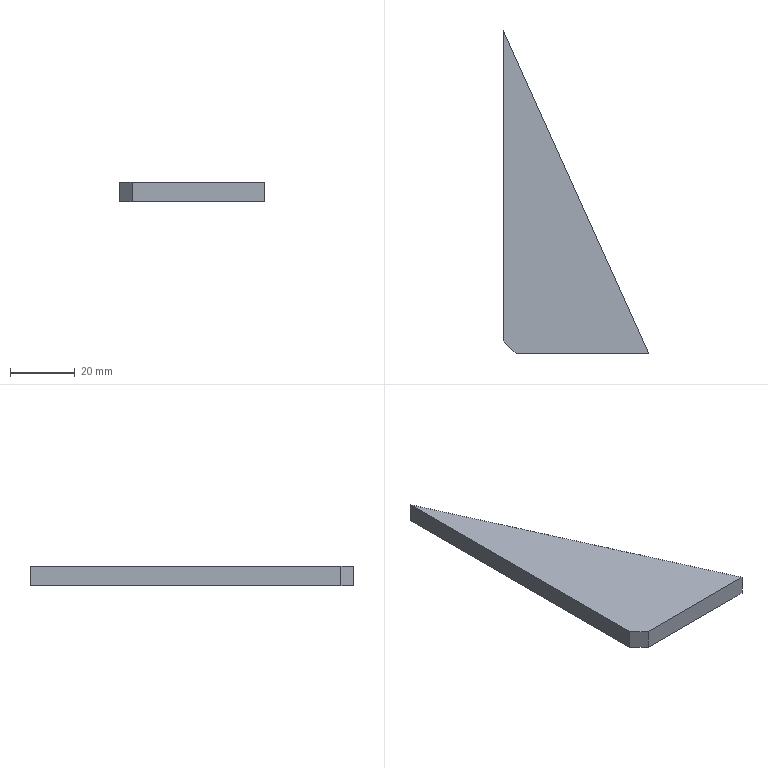Part | STEP file | BCC3 H14_6B | 1 solid | 6 faces | box 45 x 100 x 6 mm | volume 13452 mm3 | plane 6
STEP:
#1=CARTESIAN_POINT('',(0.,0.,0.));
#2=DIRECTION('',(0.,0.,1.));
#3=DIRECTION('',(1.,0.,0.));
#4=AXIS2_PLACEMENT_3D('',#1,#2,#3);
#5=CARTESIAN_POINT('',(4.,0.,6.));
#6=VERTEX_POINT('',#5);
#7=CARTESIAN_POINT('',(45.,0.,6.));
#8=VERTEX_POINT('',#7);
#9=CARTESIAN_POINT('',(45.,0.,6.));
#10=DIRECTION('',(1.,0.,0.));
#11=VECTOR('',#10,1.);
#12=LINE('',#9,#11);
#13=CARTESIAN_POINT('',(45.,0.,6.));
#14=DIRECTION('',(0.,1.,0.));
#15=DIRECTION('',(-1.,0.,0.));
#16=AXIS2_PLACEMENT_3D('',#13,#14,#15);
#17=PLANE('',#16);
#18=CARTESIAN_POINT('',(0.,0.));
#19=DIRECTION('',(-1.,0.));
#20=VECTOR('',#19,1.);
#21=LINE('',#18,#20);
#22=(GEOMETRIC_REPRESENTATION_CONTEXT(2)PARAMETRIC_REPRESENTATION_CONTEXT()REPRESENTATION_CONTEXT('',''));
#23=DEFINITIONAL_REPRESENTATION('',(#21),#22);
#24=PCURVE('',#17,#23);
#25=CARTESIAN_POINT('',(0.,0.,6.));
#26=DIRECTION('',(0.,0.,-1.));
#27=DIRECTION('',(-1.,0.,0.));
#28=AXIS2_PLACEMENT_3D('',#25,#26,#27);
#29=PLANE('',#28);
#30=CARTESIAN_POINT('',(-45.,0.));
#31=DIRECTION('',(-1.,0.));
#32=VECTOR('',#31,1.);
#33=LINE('',#30,#32);
#34=(GEOMETRIC_REPRESENTATION_CONTEXT(2)PARAMETRIC_REPRESENTATION_CONTEXT()REPRESENTATION_CONTEXT('',''));
#35=DEFINITIONAL_REPRESENTATION('',(#33),#34);
#36=PCURVE('',#29,#35);
#37=SURFACE_CURVE('',#12,(#24,#36),.PCURVE_S1.);
#38=EDGE_CURVE('',#6,#8,#37,.T.);
#39=ORIENTED_EDGE('',*,*,#38,.F.);
#40=CARTESIAN_POINT('',(4.,0.,0.));
#41=VERTEX_POINT('',#40);
#42=CARTESIAN_POINT('',(4.,0.,6.));
#43=DIRECTION('',(0.,0.,-1.));
#44=VECTOR('',#43,1.);
#45=LINE('',#42,#44);
#46=CARTESIAN_POINT('',(41.,0.));
#47=DIRECTION('',(0.,-1.));
#48=VECTOR('',#47,1.);
#49=LINE('',#46,#48);
#50=(GEOMETRIC_REPRESENTATION_CONTEXT(2)PARAMETRIC_REPRESENTATION_CONTEXT()REPRESENTATION_CONTEXT('',''));
#51=DEFINITIONAL_REPRESENTATION('',(#49),#50);
#52=PCURVE('',#17,#51);
#53=CARTESIAN_POINT('',(4.,0.,6.));
#54=DIRECTION('',(0.7071,0.7071,0.));
#55=DIRECTION('',(0.,0.,-1.));
#56=AXIS2_PLACEMENT_3D('',#53,#54,#55);
#57=PLANE('',#56);
#58=CARTESIAN_POINT('',(0.,0.));
#59=DIRECTION('',(1.,0.));
#60=VECTOR('',#59,1.);
#61=LINE('',#58,#60);
#62=(GEOMETRIC_REPRESENTATION_CONTEXT(2)PARAMETRIC_REPRESENTATION_CONTEXT()REPRESENTATION_CONTEXT('',''));
#63=DEFINITIONAL_REPRESENTATION('',(#61),#62);
#64=PCURVE('',#57,#63);
#65=SURFACE_CURVE('',#45,(#52,#64),.PCURVE_S1.);
#66=EDGE_CURVE('',#6,#41,#65,.T.);
#67=ORIENTED_EDGE('',*,*,#66,.T.);
#68=CARTESIAN_POINT('',(45.,0.,0.));
#69=VERTEX_POINT('',#68);
#70=CARTESIAN_POINT('',(45.,0.,0.));
#71=DIRECTION('',(1.,0.,0.));
#72=VECTOR('',#71,1.);
#73=LINE('',#70,#72);
#74=CARTESIAN_POINT('',(0.,-6.));
#75=DIRECTION('',(-1.,0.));
#76=VECTOR('',#75,1.);
#77=LINE('',#74,#76);
#78=(GEOMETRIC_REPRESENTATION_CONTEXT(2)PARAMETRIC_REPRESENTATION_CONTEXT()REPRESENTATION_CONTEXT('',''));
#79=DEFINITIONAL_REPRESENTATION('',(#77),#78);
#80=PCURVE('',#17,#79);
#81=CARTESIAN_POINT('',(0.,0.,0.));
#82=DIRECTION('',(0.,0.,-1.));
#83=DIRECTION('',(-1.,0.,0.));
#84=AXIS2_PLACEMENT_3D('',#81,#82,#83);
#85=PLANE('',#84);
#86=CARTESIAN_POINT('',(-45.,0.));
#87=DIRECTION('',(-1.,0.));
#88=VECTOR('',#87,1.);
#89=LINE('',#86,#88);
#90=(GEOMETRIC_REPRESENTATION_CONTEXT(2)PARAMETRIC_REPRESENTATION_CONTEXT()REPRESENTATION_CONTEXT('',''));
#91=DEFINITIONAL_REPRESENTATION('',(#89),#90);
#92=PCURVE('',#85,#91);
#93=SURFACE_CURVE('',#73,(#80,#92),.PCURVE_S1.);
#94=EDGE_CURVE('',#41,#69,#93,.T.);
#95=ORIENTED_EDGE('',*,*,#94,.T.);
#96=CARTESIAN_POINT('',(45.,0.,6.));
#97=DIRECTION('',(0.,0.,-1.));
#98=VECTOR('',#97,1.);
#99=LINE('',#96,#98);
#100=CARTESIAN_POINT('',(0.,0.));
#101=DIRECTION('',(0.,-1.));
#102=VECTOR('',#101,1.);
#103=LINE('',#100,#102);
#104=(GEOMETRIC_REPRESENTATION_CONTEXT(2)PARAMETRIC_REPRESENTATION_CONTEXT()REPRESENTATION_CONTEXT('',''));
#105=DEFINITIONAL_REPRESENTATION('',(#103),#104);
#106=PCURVE('',#17,#105);
#107=CARTESIAN_POINT('',(0.,100.,6.));
#108=DIRECTION('',(-0.9119,-0.4104,0.));
#109=DIRECTION('',(0.4104,-0.9119,0.));
#110=AXIS2_PLACEMENT_3D('',#107,#108,#109);
#111=PLANE('',#110);
#112=CARTESIAN_POINT('',(109.659,0.));
#113=DIRECTION('',(0.,-1.));
#114=VECTOR('',#113,1.);
#115=LINE('',#112,#114);
#116=(GEOMETRIC_REPRESENTATION_CONTEXT(2)PARAMETRIC_REPRESENTATION_CONTEXT()REPRESENTATION_CONTEXT('',''));
#117=DEFINITIONAL_REPRESENTATION('',(#115),#116);
#118=PCURVE('',#111,#117);
#119=SURFACE_CURVE('',#99,(#106,#118),.PCURVE_S1.);
#120=EDGE_CURVE('',#8,#69,#119,.T.);
#121=ORIENTED_EDGE('',*,*,#120,.F.);
#122=EDGE_LOOP('',(#39,#67,#95,#121));
#123=FACE_BOUND('',#122,.T.);
#124=ADVANCED_FACE('',(#123),#17,.F.);
#125=CARTESIAN_POINT('',(0.,100.,0.));
#126=VERTEX_POINT('',#125);
#127=CARTESIAN_POINT('',(0.,100.,0.));
#128=DIRECTION('',(-0.4104,0.9119,0.));
#129=VECTOR('',#128,1.);
#130=LINE('',#127,#129);
#131=CARTESIAN_POINT('',(0.,-6.));
#132=DIRECTION('',(-1.,0.));
#133=VECTOR('',#132,1.);
#134=LINE('',#131,#133);
#135=(GEOMETRIC_REPRESENTATION_CONTEXT(2)PARAMETRIC_REPRESENTATION_CONTEXT()REPRESENTATION_CONTEXT('',''));
#136=DEFINITIONAL_REPRESENTATION('',(#134),#135);
#137=PCURVE('',#111,#136);
#138=CARTESIAN_POINT('',(0.,100.));
#139=DIRECTION('',(0.4104,0.9119));
#140=VECTOR('',#139,1.);
#141=LINE('',#138,#140);
#142=(GEOMETRIC_REPRESENTATION_CONTEXT(2)PARAMETRIC_REPRESENTATION_CONTEXT()REPRESENTATION_CONTEXT('',''));
#143=DEFINITIONAL_REPRESENTATION('',(#141),#142);
#144=PCURVE('',#85,#143);
#145=SURFACE_CURVE('',#130,(#137,#144),.PCURVE_S1.);
#146=EDGE_CURVE('',#69,#126,#145,.T.);
#147=ORIENTED_EDGE('',*,*,#146,.T.);
#148=CARTESIAN_POINT('',(0.,100.,6.));
#149=VERTEX_POINT('',#148);
#150=CARTESIAN_POINT('',(0.,100.,6.));
#151=DIRECTION('',(0.,0.,-1.));
#152=VECTOR('',#151,1.);
#153=LINE('',#150,#152);
#154=CARTESIAN_POINT('',(0.,0.));
#155=DIRECTION('',(0.,-1.));
#156=VECTOR('',#155,1.);
#157=LINE('',#154,#156);
#158=(GEOMETRIC_REPRESENTATION_CONTEXT(2)PARAMETRIC_REPRESENTATION_CONTEXT()REPRESENTATION_CONTEXT('',''));
#159=DEFINITIONAL_REPRESENTATION('',(#157),#158);
#160=PCURVE('',#111,#159);
#161=CARTESIAN_POINT('',(0.,0.,6.));
#162=DIRECTION('',(1.,0.,0.));
#163=DIRECTION('',(0.,0.,-1.));
#164=AXIS2_PLACEMENT_3D('',#161,#162,#163);
#165=PLANE('',#164);
#166=CARTESIAN_POINT('',(0.,100.));
#167=DIRECTION('',(1.,0.));
#168=VECTOR('',#167,1.);
#169=LINE('',#166,#168);
#170=(GEOMETRIC_REPRESENTATION_CONTEXT(2)PARAMETRIC_REPRESENTATION_CONTEXT()REPRESENTATION_CONTEXT('',''));
#171=DEFINITIONAL_REPRESENTATION('',(#169),#170);
#172=PCURVE('',#165,#171);
#173=SURFACE_CURVE('',#153,(#160,#172),.PCURVE_S1.);
#174=EDGE_CURVE('',#149,#126,#173,.T.);
#175=ORIENTED_EDGE('',*,*,#174,.F.);
#176=CARTESIAN_POINT('',(0.,100.,6.));
#177=DIRECTION('',(-0.4104,0.9119,0.));
#178=VECTOR('',#177,1.);
#179=LINE('',#176,#178);
#180=CARTESIAN_POINT('',(0.,0.));
#181=DIRECTION('',(-1.,0.));
#182=VECTOR('',#181,1.);
#183=LINE('',#180,#182);
#184=(GEOMETRIC_REPRESENTATION_CONTEXT(2)PARAMETRIC_REPRESENTATION_CONTEXT()REPRESENTATION_CONTEXT('',''));
#185=DEFINITIONAL_REPRESENTATION('',(#183),#184);
#186=PCURVE('',#111,#185);
#187=CARTESIAN_POINT('',(0.,100.));
#188=DIRECTION('',(0.4104,0.9119));
#189=VECTOR('',#188,1.);
#190=LINE('',#187,#189);
#191=(GEOMETRIC_REPRESENTATION_CONTEXT(2)PARAMETRIC_REPRESENTATION_CONTEXT()REPRESENTATION_CONTEXT('',''));
#192=DEFINITIONAL_REPRESENTATION('',(#190),#191);
#193=PCURVE('',#29,#192);
#194=SURFACE_CURVE('',#179,(#186,#193),.PCURVE_S1.);
#195=EDGE_CURVE('',#8,#149,#194,.T.);
#196=ORIENTED_EDGE('',*,*,#195,.F.);
#197=ORIENTED_EDGE('',*,*,#120,.T.);
#198=EDGE_LOOP('',(#147,#175,#196,#197));
#199=FACE_BOUND('',#198,.T.);
#200=ADVANCED_FACE('',(#199),#111,.F.);
#201=CARTESIAN_POINT('',(0.,4.,0.));
#202=VERTEX_POINT('',#201);
#203=CARTESIAN_POINT('',(0.,0.,0.));
#204=DIRECTION('',(0.,-1.,0.));
#205=VECTOR('',#204,1.);
#206=LINE('',#203,#205);
#207=CARTESIAN_POINT('',(6.,0.));
#208=DIRECTION('',(0.,-1.));
#209=VECTOR('',#208,1.);
#210=LINE('',#207,#209);
#211=(GEOMETRIC_REPRESENTATION_CONTEXT(2)PARAMETRIC_REPRESENTATION_CONTEXT()REPRESENTATION_CONTEXT('',''));
#212=DEFINITIONAL_REPRESENTATION('',(#210),#211);
#213=PCURVE('',#165,#212);
#214=CARTESIAN_POINT('',(0.,0.));
#215=DIRECTION('',(0.,-1.));
#216=VECTOR('',#215,1.);
#217=LINE('',#214,#216);
#218=(GEOMETRIC_REPRESENTATION_CONTEXT(2)PARAMETRIC_REPRESENTATION_CONTEXT()REPRESENTATION_CONTEXT('',''));
#219=DEFINITIONAL_REPRESENTATION('',(#217),#218);
#220=PCURVE('',#85,#219);
#221=SURFACE_CURVE('',#206,(#213,#220),.PCURVE_S1.);
#222=EDGE_CURVE('',#126,#202,#221,.T.);
#223=ORIENTED_EDGE('',*,*,#222,.T.);
#224=CARTESIAN_POINT('',(0.,4.,6.));
#225=VERTEX_POINT('',#224);
#226=CARTESIAN_POINT('',(0.,4.,6.));
#227=DIRECTION('',(0.,0.,1.));
#228=VECTOR('',#227,1.);
#229=LINE('',#226,#228);
#230=CARTESIAN_POINT('',(0.,4.));
#231=DIRECTION('',(-1.,0.));
#232=VECTOR('',#231,1.);
#233=LINE('',#230,#232);
#234=(GEOMETRIC_REPRESENTATION_CONTEXT(2)PARAMETRIC_REPRESENTATION_CONTEXT()REPRESENTATION_CONTEXT('',''));
#235=DEFINITIONAL_REPRESENTATION('',(#233),#234);
#236=PCURVE('',#165,#235);
#237=CARTESIAN_POINT('',(0.,5.657));
#238=DIRECTION('',(-1.,0.));
#239=VECTOR('',#238,1.);
#240=LINE('',#237,#239);
#241=(GEOMETRIC_REPRESENTATION_CONTEXT(2)PARAMETRIC_REPRESENTATION_CONTEXT()REPRESENTATION_CONTEXT('',''));
#242=DEFINITIONAL_REPRESENTATION('',(#240),#241);
#243=PCURVE('',#57,#242);
#244=SURFACE_CURVE('',#229,(#236,#243),.PCURVE_S1.);
#245=EDGE_CURVE('',#202,#225,#244,.T.);
#246=ORIENTED_EDGE('',*,*,#245,.T.);
#247=CARTESIAN_POINT('',(0.,0.,6.));
#248=DIRECTION('',(0.,-1.,0.));
#249=VECTOR('',#248,1.);
#250=LINE('',#247,#249);
#251=CARTESIAN_POINT('',(0.,0.));
#252=DIRECTION('',(0.,-1.));
#253=VECTOR('',#252,1.);
#254=LINE('',#251,#253);
#255=(GEOMETRIC_REPRESENTATION_CONTEXT(2)PARAMETRIC_REPRESENTATION_CONTEXT()REPRESENTATION_CONTEXT('',''));
#256=DEFINITIONAL_REPRESENTATION('',(#254),#255);
#257=PCURVE('',#165,#256);
#258=CARTESIAN_POINT('',(0.,0.));
#259=DIRECTION('',(0.,-1.));
#260=VECTOR('',#259,1.);
#261=LINE('',#258,#260);
#262=(GEOMETRIC_REPRESENTATION_CONTEXT(2)PARAMETRIC_REPRESENTATION_CONTEXT()REPRESENTATION_CONTEXT('',''));
#263=DEFINITIONAL_REPRESENTATION('',(#261),#262);
#264=PCURVE('',#29,#263);
#265=SURFACE_CURVE('',#250,(#257,#264),.PCURVE_S1.);
#266=EDGE_CURVE('',#149,#225,#265,.T.);
#267=ORIENTED_EDGE('',*,*,#266,.F.);
#268=ORIENTED_EDGE('',*,*,#174,.T.);
#269=EDGE_LOOP('',(#223,#246,#267,#268));
#270=FACE_BOUND('',#269,.T.);
#271=ADVANCED_FACE('',(#270),#165,.F.);
#272=ORIENTED_EDGE('',*,*,#266,.T.);
#273=CARTESIAN_POINT('',(4.,0.,6.));
#274=DIRECTION('',(0.7071,-0.7071,0.));
#275=VECTOR('',#274,1.);
#276=LINE('',#273,#275);
#277=CARTESIAN_POINT('',(-4.,0.));
#278=DIRECTION('',(-0.7071,-0.7071));
#279=VECTOR('',#278,1.);
#280=LINE('',#277,#279);
#281=(GEOMETRIC_REPRESENTATION_CONTEXT(2)PARAMETRIC_REPRESENTATION_CONTEXT()REPRESENTATION_CONTEXT('',''));
#282=DEFINITIONAL_REPRESENTATION('',(#280),#281);
#283=PCURVE('',#29,#282);
#284=CARTESIAN_POINT('',(0.,0.));
#285=DIRECTION('',(0.,-1.));
#286=VECTOR('',#285,1.);
#287=LINE('',#284,#286);
#288=(GEOMETRIC_REPRESENTATION_CONTEXT(2)PARAMETRIC_REPRESENTATION_CONTEXT()REPRESENTATION_CONTEXT('',''));
#289=DEFINITIONAL_REPRESENTATION('',(#287),#288);
#290=PCURVE('',#57,#289);
#291=SURFACE_CURVE('',#276,(#283,#290),.PCURVE_S1.);
#292=EDGE_CURVE('',#225,#6,#291,.T.);
#293=ORIENTED_EDGE('',*,*,#292,.T.);
#294=ORIENTED_EDGE('',*,*,#38,.T.);
#295=ORIENTED_EDGE('',*,*,#195,.T.);
#296=EDGE_LOOP('',(#272,#293,#294,#295));
#297=FACE_BOUND('',#296,.T.);
#298=ADVANCED_FACE('',(#297),#29,.F.);
#299=ORIENTED_EDGE('',*,*,#94,.F.);
#300=CARTESIAN_POINT('',(2.,2.,0.));
#301=DIRECTION('',(-0.7071,0.7071,0.));
#302=VECTOR('',#301,1.);
#303=LINE('',#300,#302);
#304=CARTESIAN_POINT('',(-2.,2.));
#305=DIRECTION('',(0.7071,0.7071));
#306=VECTOR('',#305,1.);
#307=LINE('',#304,#306);
#308=(GEOMETRIC_REPRESENTATION_CONTEXT(2)PARAMETRIC_REPRESENTATION_CONTEXT()REPRESENTATION_CONTEXT('',''));
#309=DEFINITIONAL_REPRESENTATION('',(#307),#308);
#310=PCURVE('',#85,#309);
#311=CARTESIAN_POINT('',(6.,2.828));
#312=DIRECTION('',(0.,1.));
#313=VECTOR('',#312,1.);
#314=LINE('',#311,#313);
#315=(GEOMETRIC_REPRESENTATION_CONTEXT(2)PARAMETRIC_REPRESENTATION_CONTEXT()REPRESENTATION_CONTEXT('',''));
#316=DEFINITIONAL_REPRESENTATION('',(#314),#315);
#317=PCURVE('',#57,#316);
#318=SURFACE_CURVE('',#303,(#310,#317),.PCURVE_S1.);
#319=EDGE_CURVE('',#41,#202,#318,.T.);
#320=ORIENTED_EDGE('',*,*,#319,.T.);
#321=ORIENTED_EDGE('',*,*,#222,.F.);
#322=ORIENTED_EDGE('',*,*,#146,.F.);
#323=EDGE_LOOP('',(#299,#320,#321,#322));
#324=FACE_BOUND('',#323,.T.);
#325=ADVANCED_FACE('',(#324),#85,.T.);
#326=ORIENTED_EDGE('',*,*,#292,.F.);
#327=ORIENTED_EDGE('',*,*,#245,.F.);
#328=ORIENTED_EDGE('',*,*,#319,.F.);
#329=ORIENTED_EDGE('',*,*,#66,.F.);
#330=EDGE_LOOP('',(#326,#327,#328,#329));
#331=FACE_BOUND('',#330,.T.);
#332=ADVANCED_FACE('',(#331),#57,.F.);
#333=CLOSED_SHELL('',(#124,#200,#271,#298,#325,#332));
#334=MANIFOLD_SOLID_BREP('',#333);
#335=(LENGTH_UNIT()NAMED_UNIT(*)SI_UNIT(.MILLI.,.METRE.));
#336=UNCERTAINTY_MEASURE_WITH_UNIT(LENGTH_MEASURE(0.0000001),#335,'','');
#337=(NAMED_UNIT(*)PLANE_ANGLE_UNIT()SI_UNIT($,.RADIAN.));
#338=(NAMED_UNIT(*)SI_UNIT($,.STERADIAN.)SOLID_ANGLE_UNIT());
#339=(GEOMETRIC_REPRESENTATION_CONTEXT(3)GLOBAL_UNCERTAINTY_ASSIGNED_CONTEXT((#336))GLOBAL_UNIT_ASSIGNED_CONTEXT((#335,#337,#338))REPRESENTATION_CONTEXT('',''));
#340=ADVANCED_BREP_SHAPE_REPRESENTATION('',(#4,#334),#339);